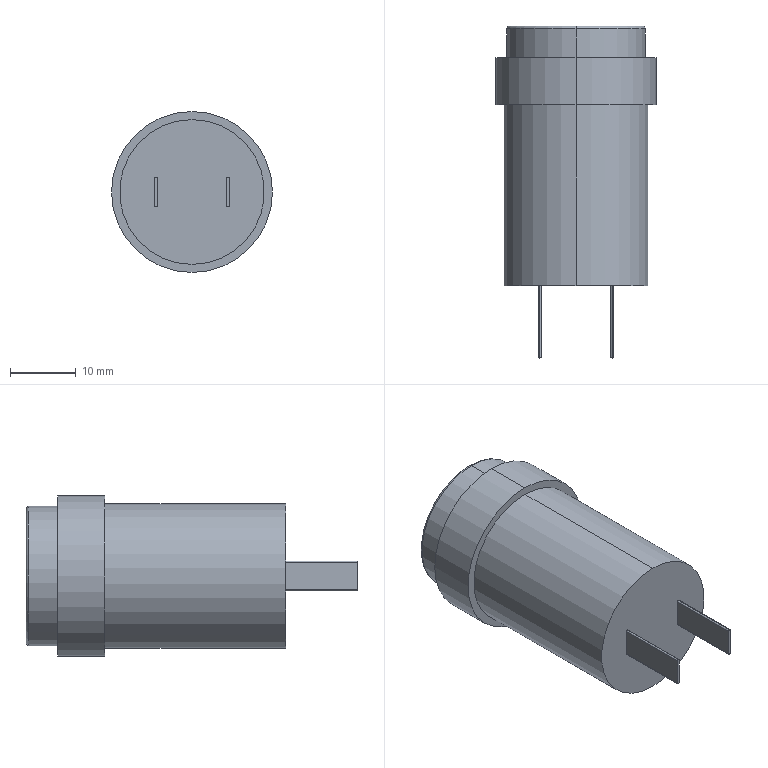Part | SolidWorks | features BaseBody 1 | 1 solid | 24 faces | box 24.475 x 50.463 x 24.475 mm | volume 15550 mm3 | cylinder 12 | plane 10 | torus 2 | commonest cylinder face diameters 0.412 x4 0.413 x2 21.175 x2 22 x2 24.475 x2
STEP:
#1=CARTESIAN_POINT('',(0.,13.6,-10.588));
#2=VERTEX_POINT('',#1);
#3=CARTESIAN_POINT('',(0.,13.6,10.588));
#4=VERTEX_POINT('',#3);
#5=CARTESIAN_POINT('',(0.,13.6,0.));
#6=DIRECTION('',(0.,-1.,0.));
#7=DIRECTION('',(0.,0.,1.));
#8=AXIS2_PLACEMENT_3D('',#5,#6,#7);
#9=CIRCLE('',#8,10.588);
#10=EDGE_CURVE('',#2,#4,#9,.T.);
#11=ORIENTED_EDGE('',*,*,#10,.F.);
#12=CARTESIAN_POINT('',(0.,14.012,-10.175));
#13=VERTEX_POINT('',#12);
#14=CARTESIAN_POINT('',(0.,13.6,-10.175));
#15=DIRECTION('',(1.,0.,0.));
#16=DIRECTION('',(0.,0.,-1.));
#17=AXIS2_PLACEMENT_3D('',#14,#15,#16);
#18=CIRCLE('',#17,0.4125);
#19=EDGE_CURVE('',#2,#13,#18,.T.);
#20=ORIENTED_EDGE('',*,*,#19,.T.);
#21=CARTESIAN_POINT('',(0.,14.012,10.175));
#22=VERTEX_POINT('',#21);
#23=CARTESIAN_POINT('',(0.,14.012,0.));
#24=DIRECTION('',(0.,1.,0.));
#25=DIRECTION('',(0.,0.,1.));
#26=AXIS2_PLACEMENT_3D('',#23,#24,#25);
#27=CIRCLE('',#26,10.175);
#28=EDGE_CURVE('',#22,#13,#27,.T.);
#29=ORIENTED_EDGE('',*,*,#28,.F.);
#30=CARTESIAN_POINT('',(0.,13.6,10.175));
#31=DIRECTION('',(-1.,0.,0.));
#32=DIRECTION('',(0.,0.,1.));
#33=AXIS2_PLACEMENT_3D('',#30,#31,#32);
#34=CIRCLE('',#33,0.4125);
#35=EDGE_CURVE('',#4,#22,#34,.T.);
#36=ORIENTED_EDGE('',*,*,#35,.F.);
#37=EDGE_LOOP('',(#11,#20,#29,#36));
#38=FACE_OUTER_BOUND('',#37,.T.);
#39=CARTESIAN_POINT('',(0.,13.6,0.));
#40=DIRECTION('',(0.,1.,0.));
#41=DIRECTION('',(0.,0.,1.));
#42=AXIS2_PLACEMENT_3D('',#39,#40,#41);
#43=TOROIDAL_SURFACE('',#42,10.175,0.4125);
#44=ADVANCED_FACE('',(#38),#43,.T.);
#45=ORIENTED_EDGE('',*,*,#10,.T.);
#46=CARTESIAN_POINT('',(0.,9.2,10.588));
#47=VERTEX_POINT('',#46);
#48=CARTESIAN_POINT('',(0.,14.012,10.588));
#49=DIRECTION('',(0.,-1.,0.));
#50=VECTOR('',#49,1000.);
#51=LINE('',#48,#50);
#52=EDGE_CURVE('',#4,#47,#51,.T.);
#53=ORIENTED_EDGE('',*,*,#52,.T.);
#54=CARTESIAN_POINT('',(0.,9.2,-10.588));
#55=VERTEX_POINT('',#54);
#56=CARTESIAN_POINT('',(0.,9.2,0.));
#57=DIRECTION('',(0.,1.,0.));
#58=DIRECTION('',(0.,0.,1.));
#59=AXIS2_PLACEMENT_3D('',#56,#57,#58);
#60=CIRCLE('',#59,10.588);
#61=EDGE_CURVE('',#47,#55,#60,.T.);
#62=ORIENTED_EDGE('',*,*,#61,.T.);
#63=CARTESIAN_POINT('',(0.,14.012,-10.588));
#64=DIRECTION('',(0.,-1.,0.));
#65=VECTOR('',#64,1000.);
#66=LINE('',#63,#65);
#67=EDGE_CURVE('',#2,#55,#66,.T.);
#68=ORIENTED_EDGE('',*,*,#67,.F.);
#69=EDGE_LOOP('',(#45,#53,#62,#68));
#70=FACE_OUTER_BOUND('',#69,.T.);
#71=CARTESIAN_POINT('',(0.,14.012,0.));
#72=DIRECTION('',(0.,-1.,0.));
#73=DIRECTION('',(0.,0.,-1.));
#74=AXIS2_PLACEMENT_3D('',#71,#72,#73);
#75=CYLINDRICAL_SURFACE('',#74,10.588);
#76=ADVANCED_FACE('',(#70),#75,.T.);
#77=CARTESIAN_POINT('',(-5.5,-36.45,2.269));
#78=VERTEX_POINT('',#77);
#79=CARTESIAN_POINT('',(-5.706,-36.45,2.062));
#80=VERTEX_POINT('',#79);
#81=CARTESIAN_POINT('',(-5.5,-36.45,2.062));
#82=DIRECTION('',(0.,-1.,0.));
#83=DIRECTION('',(0.,0.,-1.));
#84=AXIS2_PLACEMENT_3D('',#81,#82,#83);
#85=CIRCLE('',#84,0.2063);
#86=EDGE_CURVE('',#78,#80,#85,.T.);
#87=ORIENTED_EDGE('',*,*,#86,.F.);
#88=CARTESIAN_POINT('',(-5.5,-25.45,2.269));
#89=VERTEX_POINT('',#88);
#90=CARTESIAN_POINT('',(-5.5,-36.45,2.269));
#91=DIRECTION('',(0.,1.,0.));
#92=VECTOR('',#91,1000.);
#93=LINE('',#90,#92);
#94=EDGE_CURVE('',#78,#89,#93,.T.);
#95=ORIENTED_EDGE('',*,*,#94,.T.);
#96=CARTESIAN_POINT('',(-5.706,-25.45,2.062));
#97=VERTEX_POINT('',#96);
#98=CARTESIAN_POINT('',(-5.5,-25.45,2.062));
#99=DIRECTION('',(0.,-1.,0.));
#100=DIRECTION('',(0.,0.,-1.));
#101=AXIS2_PLACEMENT_3D('',#98,#99,#100);
#102=CIRCLE('',#101,0.2063);
#103=EDGE_CURVE('',#89,#97,#102,.T.);
#104=ORIENTED_EDGE('',*,*,#103,.T.);
#105=CARTESIAN_POINT('',(-5.706,-36.45,2.062));
#106=DIRECTION('',(0.,1.,0.));
#107=VECTOR('',#106,1000.);
#108=LINE('',#105,#107);
#109=EDGE_CURVE('',#80,#97,#108,.T.);
#110=ORIENTED_EDGE('',*,*,#109,.F.);
#111=EDGE_LOOP('',(#87,#95,#104,#110));
#112=FACE_OUTER_BOUND('',#111,.T.);
#113=CARTESIAN_POINT('',(-5.5,-36.45,2.062));
#114=DIRECTION('',(0.,1.,0.));
#115=DIRECTION('',(0.,0.,1.));
#116=AXIS2_PLACEMENT_3D('',#113,#114,#115);
#117=CYLINDRICAL_SURFACE('',#116,0.2062);
#118=ADVANCED_FACE('',(#112),#117,.T.);
#119=CARTESIAN_POINT('',(5.5,-36.45,2.269));
#120=VERTEX_POINT('',#119);
#121=CARTESIAN_POINT('',(5.294,-36.45,2.062));
#122=VERTEX_POINT('',#121);
#123=CARTESIAN_POINT('',(5.5,-36.45,2.062));
#124=DIRECTION('',(0.,-1.,0.));
#125=DIRECTION('',(0.,0.,-1.));
#126=AXIS2_PLACEMENT_3D('',#123,#124,#125);
#127=CIRCLE('',#126,0.2063);
#128=EDGE_CURVE('',#120,#122,#127,.T.);
#129=ORIENTED_EDGE('',*,*,#128,.F.);
#130=CARTESIAN_POINT('',(5.5,-25.45,2.269));
#131=VERTEX_POINT('',#130);
#132=CARTESIAN_POINT('',(5.5,-36.45,2.269));
#133=DIRECTION('',(0.,1.,0.));
#134=VECTOR('',#133,1000.);
#135=LINE('',#132,#134);
#136=EDGE_CURVE('',#120,#131,#135,.T.);
#137=ORIENTED_EDGE('',*,*,#136,.T.);
#138=CARTESIAN_POINT('',(5.294,-25.45,2.062));
#139=VERTEX_POINT('',#138);
#140=CARTESIAN_POINT('',(5.5,-25.45,2.062));
#141=DIRECTION('',(0.,-1.,0.));
#142=DIRECTION('',(0.,0.,-1.));
#143=AXIS2_PLACEMENT_3D('',#140,#141,#142);
#144=CIRCLE('',#143,0.2063);
#145=EDGE_CURVE('',#131,#139,#144,.T.);
#146=ORIENTED_EDGE('',*,*,#145,.T.);
#147=CARTESIAN_POINT('',(5.294,-36.45,2.062));
#148=DIRECTION('',(0.,1.,0.));
#149=VECTOR('',#148,1000.);
#150=LINE('',#147,#149);
#151=EDGE_CURVE('',#122,#139,#150,.T.);
#152=ORIENTED_EDGE('',*,*,#151,.F.);
#153=EDGE_LOOP('',(#129,#137,#146,#152));
#154=FACE_OUTER_BOUND('',#153,.T.);
#155=CARTESIAN_POINT('',(5.5,-36.45,2.062));
#156=DIRECTION('',(0.,1.,0.));
#157=DIRECTION('',(0.,0.,1.));
#158=AXIS2_PLACEMENT_3D('',#155,#156,#157);
#159=CYLINDRICAL_SURFACE('',#158,0.2062);
#160=ADVANCED_FACE('',(#154),#159,.T.);
#161=CARTESIAN_POINT('',(0.,-25.45,-11.));
#162=VERTEX_POINT('',#161);
#163=CARTESIAN_POINT('',(0.,-25.45,11.));
#164=VERTEX_POINT('',#163);
#165=CARTESIAN_POINT('',(0.,-25.45,0.));
#166=DIRECTION('',(0.,-1.,0.));
#167=DIRECTION('',(0.,0.,-1.));
#168=AXIS2_PLACEMENT_3D('',#165,#166,#167);
#169=CIRCLE('',#168,11.);
#170=EDGE_CURVE('',#162,#164,#169,.T.);
#171=ORIENTED_EDGE('',*,*,#170,.F.);
#172=CARTESIAN_POINT('',(0.,2.05,-11.));
#173=VERTEX_POINT('',#172);
#174=CARTESIAN_POINT('',(0.,-25.45,-11.));
#175=DIRECTION('',(0.,1.,0.));
#176=VECTOR('',#175,1000.);
#177=LINE('',#174,#176);
#178=EDGE_CURVE('',#162,#173,#177,.T.);
#179=ORIENTED_EDGE('',*,*,#178,.T.);
#180=CARTESIAN_POINT('',(0.,2.05,11.));
#181=VERTEX_POINT('',#180);
#182=CARTESIAN_POINT('',(0.,2.05,0.));
#183=DIRECTION('',(0.,-1.,0.));
#184=DIRECTION('',(0.,0.,1.));
#185=AXIS2_PLACEMENT_3D('',#182,#183,#184);
#186=CIRCLE('',#185,11.);
#187=EDGE_CURVE('',#173,#181,#186,.T.);
#188=ORIENTED_EDGE('',*,*,#187,.T.);
#189=CARTESIAN_POINT('',(0.,-25.45,11.));
#190=DIRECTION('',(0.,1.,0.));
#191=VECTOR('',#190,1000.);
#192=LINE('',#189,#191);
#193=EDGE_CURVE('',#164,#181,#192,.T.);
#194=ORIENTED_EDGE('',*,*,#193,.F.);
#195=EDGE_LOOP('',(#171,#179,#188,#194));
#196=FACE_OUTER_BOUND('',#195,.T.);
#197=CARTESIAN_POINT('',(0.,-25.45,0.));
#198=DIRECTION('',(0.,1.,0.));
#199=DIRECTION('',(0.,0.,1.));
#200=AXIS2_PLACEMENT_3D('',#197,#198,#199);
#201=CYLINDRICAL_SURFACE('',#200,11.);
#202=ADVANCED_FACE('',(#196),#201,.T.);
#203=CARTESIAN_POINT('',(0.,9.2,12.238));
#204=VERTEX_POINT('',#203);
#205=CARTESIAN_POINT('',(0.,9.2,-12.238));
#206=VERTEX_POINT('',#205);
#207=CARTESIAN_POINT('',(0.,9.2,0.));
#208=DIRECTION('',(0.,1.,0.));
#209=DIRECTION('',(0.,0.,1.));
#210=AXIS2_PLACEMENT_3D('',#207,#208,#209);
#211=CIRCLE('',#210,12.238);
#212=EDGE_CURVE('',#204,#206,#211,.T.);
#213=ORIENTED_EDGE('',*,*,#212,.F.);
#214=CARTESIAN_POINT('',(0.,2.05,12.238));
#215=VERTEX_POINT('',#214);
#216=CARTESIAN_POINT('',(0.,9.2,12.238));
#217=DIRECTION('',(0.,-1.,0.));
#218=VECTOR('',#217,1000.);
#219=LINE('',#216,#218);
#220=EDGE_CURVE('',#204,#215,#219,.T.);
#221=ORIENTED_EDGE('',*,*,#220,.T.);
#222=CARTESIAN_POINT('',(0.,2.05,-12.238));
#223=VERTEX_POINT('',#222);
#224=CARTESIAN_POINT('',(0.,2.05,0.));
#225=DIRECTION('',(0.,1.,0.));
#226=DIRECTION('',(0.,0.,1.));
#227=AXIS2_PLACEMENT_3D('',#224,#225,#226);
#228=CIRCLE('',#227,12.238);
#229=EDGE_CURVE('',#215,#223,#228,.T.);
#230=ORIENTED_EDGE('',*,*,#229,.T.);
#231=CARTESIAN_POINT('',(0.,9.2,-12.238));
#232=DIRECTION('',(0.,-1.,0.));
#233=VECTOR('',#232,1000.);
#234=LINE('',#231,#233);
#235=EDGE_CURVE('',#206,#223,#234,.T.);
#236=ORIENTED_EDGE('',*,*,#235,.F.);
#237=EDGE_LOOP('',(#213,#221,#230,#236));
#238=FACE_OUTER_BOUND('',#237,.T.);
#239=CARTESIAN_POINT('',(0.,9.2,0.));
#240=DIRECTION('',(0.,-1.,0.));
#241=DIRECTION('',(0.,0.,-1.));
#242=AXIS2_PLACEMENT_3D('',#239,#240,#241);
#243=CYLINDRICAL_SURFACE('',#242,12.238);
#244=ADVANCED_FACE('',(#238),#243,.T.);
#245=CARTESIAN_POINT('',(0.,9.2,0.));
#246=DIRECTION('',(0.,1.,0.));
#247=DIRECTION('',(0.,0.,1.));
#248=AXIS2_PLACEMENT_3D('',#245,#246,#247);
#249=CIRCLE('',#248,12.238);
#250=EDGE_CURVE('',#206,#204,#249,.T.);
#251=ORIENTED_EDGE('',*,*,#250,.T.);
#252=ORIENTED_EDGE('',*,*,#212,.T.);
#253=EDGE_LOOP('',(#251,#252));
#254=FACE_OUTER_BOUND('',#253,.T.);
#255=CARTESIAN_POINT('',(0.,9.2,0.));
#256=DIRECTION('',(0.,1.,0.));
#257=DIRECTION('',(0.,0.,1.));
#258=AXIS2_PLACEMENT_3D('',#255,#256,#257);
#259=CIRCLE('',#258,10.588);
#260=EDGE_CURVE('',#55,#47,#259,.T.);
#261=ORIENTED_EDGE('',*,*,#260,.F.);
#262=ORIENTED_EDGE('',*,*,#61,.F.);
#263=EDGE_LOOP('',(#261,#262));
#264=FACE_BOUND('',#263,.T.);
#265=CARTESIAN_POINT('',(0.,9.2,0.));
#266=DIRECTION('',(0.,1.,0.));
#267=DIRECTION('',(0.,0.,1.));
#268=AXIS2_PLACEMENT_3D('',#265,#266,#267);
#269=PLANE('',#268);
#270=ADVANCED_FACE('',(#254,#264),#269,.T.);
#271=CARTESIAN_POINT('',(5.294,-25.45,-2.062));
#272=VERTEX_POINT('',#271);
#273=CARTESIAN_POINT('',(5.294,-25.45,2.062));
#274=DIRECTION('',(0.,0.,-1.));
#275=VECTOR('',#274,1000.);
#276=LINE('',#273,#275);
#277=EDGE_CURVE('',#139,#272,#276,.T.);
#278=ORIENTED_EDGE('',*,*,#277,.F.);
#279=ORIENTED_EDGE('',*,*,#145,.F.);
#280=CARTESIAN_POINT('',(5.706,-25.45,2.062));
#281=VERTEX_POINT('',#280);
#282=CARTESIAN_POINT('',(5.5,-25.45,2.062));
#283=DIRECTION('',(0.,-1.,0.));
#284=DIRECTION('',(0.,0.,-1.));
#285=AXIS2_PLACEMENT_3D('',#282,#283,#284);
#286=CIRCLE('',#285,0.2063);
#287=EDGE_CURVE('',#281,#131,#286,.T.);
#288=ORIENTED_EDGE('',*,*,#287,.F.);
#289=CARTESIAN_POINT('',(5.706,-25.45,-2.062));
#290=VERTEX_POINT('',#289);
#291=CARTESIAN_POINT('',(5.706,-25.45,2.062));
#292=DIRECTION('',(0.,0.,1.));
#293=VECTOR('',#292,1000.);
#294=LINE('',#291,#293);
#295=EDGE_CURVE('',#290,#281,#294,.T.);
#296=ORIENTED_EDGE('',*,*,#295,.F.);
#297=CARTESIAN_POINT('',(5.5,-25.45,-2.062));
#298=DIRECTION('',(0.,-1.,0.));
#299=DIRECTION('',(0.,0.,-1.));
#300=AXIS2_PLACEMENT_3D('',#297,#298,#299);
#301=CIRCLE('',#300,0.2062);
#302=EDGE_CURVE('',#272,#290,#301,.T.);
#303=ORIENTED_EDGE('',*,*,#302,.F.);
#304=EDGE_LOOP('',(#278,#279,#288,#296,#303));
#305=FACE_BOUND('',#304,.T.);
#306=CARTESIAN_POINT('',(0.,-25.45,0.));
#307=DIRECTION('',(0.,-1.,0.));
#308=DIRECTION('',(0.,0.,-1.));
#309=AXIS2_PLACEMENT_3D('',#306,#307,#308);
#310=CIRCLE('',#309,11.);
#311=EDGE_CURVE('',#164,#162,#310,.T.);
#312=ORIENTED_EDGE('',*,*,#311,.T.);
#313=ORIENTED_EDGE('',*,*,#170,.T.);
#314=EDGE_LOOP('',(#312,#313));
#315=FACE_OUTER_BOUND('',#314,.T.);
#316=CARTESIAN_POINT('',(-5.706,-25.45,-2.062));
#317=VERTEX_POINT('',#316);
#318=CARTESIAN_POINT('',(-5.706,-25.45,2.062));
#319=DIRECTION('',(0.,0.,-1.));
#320=VECTOR('',#319,1000.);
#321=LINE('',#318,#320);
#322=EDGE_CURVE('',#97,#317,#321,.T.);
#323=ORIENTED_EDGE('',*,*,#322,.F.);
#324=ORIENTED_EDGE('',*,*,#103,.F.);
#325=CARTESIAN_POINT('',(-5.294,-25.45,2.062));
#326=VERTEX_POINT('',#325);
#327=CARTESIAN_POINT('',(-5.5,-25.45,2.062));
#328=DIRECTION('',(0.,-1.,0.));
#329=DIRECTION('',(0.,0.,-1.));
#330=AXIS2_PLACEMENT_3D('',#327,#328,#329);
#331=CIRCLE('',#330,0.2063);
#332=EDGE_CURVE('',#326,#89,#331,.T.);
#333=ORIENTED_EDGE('',*,*,#332,.F.);
#334=CARTESIAN_POINT('',(-5.294,-25.45,-2.062));
#335=VERTEX_POINT('',#334);
#336=CARTESIAN_POINT('',(-5.294,-25.45,2.062));
#337=DIRECTION('',(0.,0.,1.));
#338=VECTOR('',#337,1000.);
#339=LINE('',#336,#338);
#340=EDGE_CURVE('',#335,#326,#339,.T.);
#341=ORIENTED_EDGE('',*,*,#340,.F.);
#342=CARTESIAN_POINT('',(-5.5,-25.45,-2.062));
#343=DIRECTION('',(0.,-1.,0.));
#344=DIRECTION('',(0.,0.,-1.));
#345=AXIS2_PLACEMENT_3D('',#342,#343,#344);
#346=CIRCLE('',#345,0.2062);
#347=EDGE_CURVE('',#317,#335,#346,.T.);
#348=ORIENTED_EDGE('',*,*,#347,.F.);
#349=EDGE_LOOP('',(#323,#324,#333,#341,#348));
#350=FACE_BOUND('',#349,.T.);
#351=CARTESIAN_POINT('',(0.,-25.45,0.));
#352=DIRECTION('',(0.,-1.,0.));
#353=DIRECTION('',(0.,0.,-1.));
#354=AXIS2_PLACEMENT_3D('',#351,#352,#353);
#355=PLANE('',#354);
#356=ADVANCED_FACE('',(#305,#315,#350),#355,.T.);
#357=CARTESIAN_POINT('',(0.,2.05,0.));
#358=DIRECTION('',(0.,1.,0.));
#359=DIRECTION('',(0.,0.,1.));
#360=AXIS2_PLACEMENT_3D('',#357,#358,#359);
#361=CIRCLE('',#360,12.238);
#362=EDGE_CURVE('',#223,#215,#361,.T.);
#363=ORIENTED_EDGE('',*,*,#362,.F.);
#364=ORIENTED_EDGE('',*,*,#229,.F.);
#365=EDGE_LOOP('',(#363,#364));
#366=FACE_OUTER_BOUND('',#365,.T.);
#367=CARTESIAN_POINT('',(0.,2.05,0.));
#368=DIRECTION('',(0.,-1.,0.));
#369=DIRECTION('',(0.,0.,1.));
#370=AXIS2_PLACEMENT_3D('',#367,#368,#369);
#371=CIRCLE('',#370,11.);
#372=EDGE_CURVE('',#181,#173,#371,.T.);
#373=ORIENTED_EDGE('',*,*,#372,.F.);
#374=ORIENTED_EDGE('',*,*,#187,.F.);
#375=EDGE_LOOP('',(#373,#374));
#376=FACE_BOUND('',#375,.T.);
#377=CARTESIAN_POINT('',(0.,2.05,0.));
#378=DIRECTION('',(0.,1.,0.));
#379=DIRECTION('',(0.,0.,1.));
#380=AXIS2_PLACEMENT_3D('',#377,#378,#379);
#381=PLANE('',#380);
#382=ADVANCED_FACE('',(#366,#376),#381,.F.);
#383=ORIENTED_EDGE('',*,*,#220,.F.);
#384=ORIENTED_EDGE('',*,*,#250,.F.);
#385=ORIENTED_EDGE('',*,*,#235,.T.);
#386=ORIENTED_EDGE('',*,*,#362,.T.);
#387=EDGE_LOOP('',(#383,#384,#385,#386));
#388=FACE_OUTER_BOUND('',#387,.T.);
#389=CARTESIAN_POINT('',(0.,9.2,0.));
#390=DIRECTION('',(0.,-1.,0.));
#391=DIRECTION('',(0.,0.,-1.));
#392=AXIS2_PLACEMENT_3D('',#389,#390,#391);
#393=CYLINDRICAL_SURFACE('',#392,12.238);
#394=ADVANCED_FACE('',(#388),#393,.T.);
#395=ORIENTED_EDGE('',*,*,#178,.F.);
#396=ORIENTED_EDGE('',*,*,#311,.F.);
#397=ORIENTED_EDGE('',*,*,#193,.T.);
#398=ORIENTED_EDGE('',*,*,#372,.T.);
#399=EDGE_LOOP('',(#395,#396,#397,#398));
#400=FACE_OUTER_BOUND('',#399,.T.);
#401=CARTESIAN_POINT('',(0.,-25.45,0.));
#402=DIRECTION('',(0.,1.,0.));
#403=DIRECTION('',(0.,0.,1.));
#404=AXIS2_PLACEMENT_3D('',#401,#402,#403);
#405=CYLINDRICAL_SURFACE('',#404,11.);
#406=ADVANCED_FACE('',(#400),#405,.T.);
#407=ORIENTED_EDGE('',*,*,#136,.F.);
#408=CARTESIAN_POINT('',(5.706,-36.45,2.062));
#409=VERTEX_POINT('',#408);
#410=CARTESIAN_POINT('',(5.5,-36.45,2.062));
#411=DIRECTION('',(0.,-1.,0.));
#412=DIRECTION('',(0.,0.,-1.));
#413=AXIS2_PLACEMENT_3D('',#410,#411,#412);
#414=CIRCLE('',#413,0.2063);
#415=EDGE_CURVE('',#409,#120,#414,.T.);
#416=ORIENTED_EDGE('',*,*,#415,.F.);
#417=CARTESIAN_POINT('',(5.706,-36.45,2.062));
#418=DIRECTION('',(0.,1.,0.));
#419=VECTOR('',#418,1000.);
#420=LINE('',#417,#419);
#421=EDGE_CURVE('',#409,#281,#420,.T.);
#422=ORIENTED_EDGE('',*,*,#421,.T.);
#423=ORIENTED_EDGE('',*,*,#287,.T.);
#424=EDGE_LOOP('',(#407,#416,#422,#423));
#425=FACE_OUTER_BOUND('',#424,.T.);
#426=CARTESIAN_POINT('',(5.5,-36.45,2.062));
#427=DIRECTION('',(0.,1.,0.));
#428=DIRECTION('',(0.,0.,1.));
#429=AXIS2_PLACEMENT_3D('',#426,#427,#428);
#430=CYLINDRICAL_SURFACE('',#429,0.2062);
#431=ADVANCED_FACE('',(#425),#430,.T.);
#432=ORIENTED_EDGE('',*,*,#277,.T.);
#433=CARTESIAN_POINT('',(5.294,-36.45,-2.062));
#434=VERTEX_POINT('',#433);
#435=CARTESIAN_POINT('',(5.294,-36.45,-2.062));
#436=DIRECTION('',(0.,1.,0.));
#437=VECTOR('',#436,1000.);
#438=LINE('',#435,#437);
#439=EDGE_CURVE('',#434,#272,#438,.T.);
#440=ORIENTED_EDGE('',*,*,#439,.F.);
#441=CARTESIAN_POINT('',(5.294,-36.45,2.062));
#442=DIRECTION('',(0.,0.,-1.));
#443=VECTOR('',#442,1000.);
#444=LINE('',#441,#443);
#445=EDGE_CURVE('',#122,#434,#444,.T.);
#446=ORIENTED_EDGE('',*,*,#445,.F.);
#447=ORIENTED_EDGE('',*,*,#151,.T.);
#448=EDGE_LOOP('',(#432,#440,#446,#447));
#449=FACE_OUTER_BOUND('',#448,.T.);
#450=CARTESIAN_POINT('',(5.294,-36.45,2.062));
#451=DIRECTION('',(1.,0.,0.));
#452=DIRECTION('',(0.,0.,-1.));
#453=AXIS2_PLACEMENT_3D('',#450,#451,#452);
#454=PLANE('',#453);
#455=ADVANCED_FACE('',(#449),#454,.F.);
#456=ORIENTED_EDGE('',*,*,#302,.T.);
#457=CARTESIAN_POINT('',(5.706,-36.45,-2.062));
#458=VERTEX_POINT('',#457);
#459=CARTESIAN_POINT('',(5.706,-36.45,-2.062));
#460=DIRECTION('',(0.,1.,0.));
#461=VECTOR('',#460,1000.);
#462=LINE('',#459,#461);
#463=EDGE_CURVE('',#458,#290,#462,.T.);
#464=ORIENTED_EDGE('',*,*,#463,.F.);
#465=CARTESIAN_POINT('',(5.5,-36.45,-2.062));
#466=DIRECTION('',(0.,-1.,0.));
#467=DIRECTION('',(0.,0.,-1.));
#468=AXIS2_PLACEMENT_3D('',#465,#466,#467);
#469=CIRCLE('',#468,0.2062);
#470=EDGE_CURVE('',#434,#458,#469,.T.);
#471=ORIENTED_EDGE('',*,*,#470,.F.);
#472=ORIENTED_EDGE('',*,*,#439,.T.);
#473=EDGE_LOOP('',(#456,#464,#471,#472));
#474=FACE_OUTER_BOUND('',#473,.T.);
#475=CARTESIAN_POINT('',(5.5,-36.45,-2.062));
#476=DIRECTION('',(0.,1.,0.));
#477=DIRECTION('',(0.,0.,1.));
#478=AXIS2_PLACEMENT_3D('',#475,#476,#477);
#479=CYLINDRICAL_SURFACE('',#478,0.2063);
#480=ADVANCED_FACE('',(#474),#479,.T.);
#481=ORIENTED_EDGE('',*,*,#295,.T.);
#482=ORIENTED_EDGE('',*,*,#421,.F.);
#483=CARTESIAN_POINT('',(5.706,-36.45,2.062));
#484=DIRECTION('',(0.,0.,1.));
#485=VECTOR('',#484,1000.);
#486=LINE('',#483,#485);
#487=EDGE_CURVE('',#458,#409,#486,.T.);
#488=ORIENTED_EDGE('',*,*,#487,.F.);
#489=ORIENTED_EDGE('',*,*,#463,.T.);
#490=EDGE_LOOP('',(#481,#482,#488,#489));
#491=FACE_OUTER_BOUND('',#490,.T.);
#492=CARTESIAN_POINT('',(5.706,-36.45,2.062));
#493=DIRECTION('',(-1.,0.,0.));
#494=DIRECTION('',(0.,0.,1.));
#495=AXIS2_PLACEMENT_3D('',#492,#493,#494);
#496=PLANE('',#495);
#497=ADVANCED_FACE('',(#491),#496,.F.);
#498=ORIENTED_EDGE('',*,*,#415,.T.);
#499=ORIENTED_EDGE('',*,*,#128,.T.);
#500=ORIENTED_EDGE('',*,*,#445,.T.);
#501=ORIENTED_EDGE('',*,*,#470,.T.);
#502=ORIENTED_EDGE('',*,*,#487,.T.);
#503=EDGE_LOOP('',(#498,#499,#500,#501,#502));
#504=FACE_OUTER_BOUND('',#503,.T.);
#505=CARTESIAN_POINT('',(5.5,-36.45,2.062));
#506=DIRECTION('',(0.,-1.,0.));
#507=DIRECTION('',(0.,0.,-1.));
#508=AXIS2_PLACEMENT_3D('',#505,#506,#507);
#509=PLANE('',#508);
#510=ADVANCED_FACE('',(#504),#509,.T.);
#511=ORIENTED_EDGE('',*,*,#94,.F.);
#512=CARTESIAN_POINT('',(-5.294,-36.45,2.062));
#513=VERTEX_POINT('',#512);
#514=CARTESIAN_POINT('',(-5.5,-36.45,2.062));
#515=DIRECTION('',(0.,-1.,0.));
#516=DIRECTION('',(0.,0.,-1.));
#517=AXIS2_PLACEMENT_3D('',#514,#515,#516);
#518=CIRCLE('',#517,0.2063);
#519=EDGE_CURVE('',#513,#78,#518,.T.);
#520=ORIENTED_EDGE('',*,*,#519,.F.);
#521=CARTESIAN_POINT('',(-5.294,-36.45,2.062));
#522=DIRECTION('',(0.,1.,0.));
#523=VECTOR('',#522,1000.);
#524=LINE('',#521,#523);
#525=EDGE_CURVE('',#513,#326,#524,.T.);
#526=ORIENTED_EDGE('',*,*,#525,.T.);
#527=ORIENTED_EDGE('',*,*,#332,.T.);
#528=EDGE_LOOP('',(#511,#520,#526,#527));
#529=FACE_OUTER_BOUND('',#528,.T.);
#530=CARTESIAN_POINT('',(-5.5,-36.45,2.062));
#531=DIRECTION('',(0.,1.,0.));
#532=DIRECTION('',(0.,0.,1.));
#533=AXIS2_PLACEMENT_3D('',#530,#531,#532);
#534=CYLINDRICAL_SURFACE('',#533,0.2062);
#535=ADVANCED_FACE('',(#529),#534,.T.);
#536=ORIENTED_EDGE('',*,*,#322,.T.);
#537=CARTESIAN_POINT('',(-5.706,-36.45,-2.062));
#538=VERTEX_POINT('',#537);
#539=CARTESIAN_POINT('',(-5.706,-36.45,-2.062));
#540=DIRECTION('',(0.,1.,0.));
#541=VECTOR('',#540,1000.);
#542=LINE('',#539,#541);
#543=EDGE_CURVE('',#538,#317,#542,.T.);
#544=ORIENTED_EDGE('',*,*,#543,.F.);
#545=CARTESIAN_POINT('',(-5.706,-36.45,2.062));
#546=DIRECTION('',(0.,0.,-1.));
#547=VECTOR('',#546,1000.);
#548=LINE('',#545,#547);
#549=EDGE_CURVE('',#80,#538,#548,.T.);
#550=ORIENTED_EDGE('',*,*,#549,.F.);
#551=ORIENTED_EDGE('',*,*,#109,.T.);
#552=EDGE_LOOP('',(#536,#544,#550,#551));
#553=FACE_OUTER_BOUND('',#552,.T.);
#554=CARTESIAN_POINT('',(-5.706,-36.45,2.062));
#555=DIRECTION('',(1.,0.,0.));
#556=DIRECTION('',(0.,0.,-1.));
#557=AXIS2_PLACEMENT_3D('',#554,#555,#556);
#558=PLANE('',#557);
#559=ADVANCED_FACE('',(#553),#558,.F.);
#560=ORIENTED_EDGE('',*,*,#347,.T.);
#561=CARTESIAN_POINT('',(-5.294,-36.45,-2.062));
#562=VERTEX_POINT('',#561);
#563=CARTESIAN_POINT('',(-5.294,-36.45,-2.062));
#564=DIRECTION('',(0.,1.,0.));
#565=VECTOR('',#564,1000.);
#566=LINE('',#563,#565);
#567=EDGE_CURVE('',#562,#335,#566,.T.);
#568=ORIENTED_EDGE('',*,*,#567,.F.);
#569=CARTESIAN_POINT('',(-5.5,-36.45,-2.062));
#570=DIRECTION('',(0.,-1.,0.));
#571=DIRECTION('',(0.,0.,-1.));
#572=AXIS2_PLACEMENT_3D('',#569,#570,#571);
#573=CIRCLE('',#572,0.2062);
#574=EDGE_CURVE('',#538,#562,#573,.T.);
#575=ORIENTED_EDGE('',*,*,#574,.F.);
#576=ORIENTED_EDGE('',*,*,#543,.T.);
#577=EDGE_LOOP('',(#560,#568,#575,#576));
#578=FACE_OUTER_BOUND('',#577,.T.);
#579=CARTESIAN_POINT('',(-5.5,-36.45,-2.062));
#580=DIRECTION('',(0.,1.,0.));
#581=DIRECTION('',(0.,0.,1.));
#582=AXIS2_PLACEMENT_3D('',#579,#580,#581);
#583=CYLINDRICAL_SURFACE('',#582,0.2063);
#584=ADVANCED_FACE('',(#578),#583,.T.);
#585=ORIENTED_EDGE('',*,*,#340,.T.);
#586=ORIENTED_EDGE('',*,*,#525,.F.);
#587=CARTESIAN_POINT('',(-5.294,-36.45,2.062));
#588=DIRECTION('',(0.,0.,1.));
#589=VECTOR('',#588,1000.);
#590=LINE('',#587,#589);
#591=EDGE_CURVE('',#562,#513,#590,.T.);
#592=ORIENTED_EDGE('',*,*,#591,.F.);
#593=ORIENTED_EDGE('',*,*,#567,.T.);
#594=EDGE_LOOP('',(#585,#586,#592,#593));
#595=FACE_OUTER_BOUND('',#594,.T.);
#596=CARTESIAN_POINT('',(-5.294,-36.45,2.062));
#597=DIRECTION('',(-1.,0.,0.));
#598=DIRECTION('',(0.,0.,1.));
#599=AXIS2_PLACEMENT_3D('',#596,#597,#598);
#600=PLANE('',#599);
#601=ADVANCED_FACE('',(#595),#600,.F.);
#602=ORIENTED_EDGE('',*,*,#519,.T.);
#603=ORIENTED_EDGE('',*,*,#86,.T.);
#604=ORIENTED_EDGE('',*,*,#549,.T.);
#605=ORIENTED_EDGE('',*,*,#574,.T.);
#606=ORIENTED_EDGE('',*,*,#591,.T.);
#607=EDGE_LOOP('',(#602,#603,#604,#605,#606));
#608=FACE_OUTER_BOUND('',#607,.T.);
#609=CARTESIAN_POINT('',(-5.5,-36.45,2.062));
#610=DIRECTION('',(0.,-1.,0.));
#611=DIRECTION('',(0.,0.,-1.));
#612=AXIS2_PLACEMENT_3D('',#609,#610,#611);
#613=PLANE('',#612);
#614=ADVANCED_FACE('',(#608),#613,.T.);
#615=ORIENTED_EDGE('',*,*,#52,.F.);
#616=CARTESIAN_POINT('',(0.,13.6,0.));
#617=DIRECTION('',(0.,-1.,0.));
#618=DIRECTION('',(0.,0.,1.));
#619=AXIS2_PLACEMENT_3D('',#616,#617,#618);
#620=CIRCLE('',#619,10.588);
#621=EDGE_CURVE('',#4,#2,#620,.T.);
#622=ORIENTED_EDGE('',*,*,#621,.T.);
#623=ORIENTED_EDGE('',*,*,#67,.T.);
#624=ORIENTED_EDGE('',*,*,#260,.T.);
#625=EDGE_LOOP('',(#615,#622,#623,#624));
#626=FACE_OUTER_BOUND('',#625,.T.);
#627=CARTESIAN_POINT('',(0.,14.012,0.));
#628=DIRECTION('',(0.,-1.,0.));
#629=DIRECTION('',(0.,0.,-1.));
#630=AXIS2_PLACEMENT_3D('',#627,#628,#629);
#631=CYLINDRICAL_SURFACE('',#630,10.588);
#632=ADVANCED_FACE('',(#626),#631,.T.);
#633=ORIENTED_EDGE('',*,*,#28,.T.);
#634=CARTESIAN_POINT('',(0.,14.012,0.));
#635=DIRECTION('',(0.,1.,0.));
#636=DIRECTION('',(0.,0.,1.));
#637=AXIS2_PLACEMENT_3D('',#634,#635,#636);
#638=CIRCLE('',#637,10.175);
#639=EDGE_CURVE('',#13,#22,#638,.T.);
#640=ORIENTED_EDGE('',*,*,#639,.T.);
#641=EDGE_LOOP('',(#633,#640));
#642=FACE_OUTER_BOUND('',#641,.T.);
#643=CARTESIAN_POINT('',(0.,14.012,0.));
#644=DIRECTION('',(0.,1.,0.));
#645=DIRECTION('',(0.,0.,1.));
#646=AXIS2_PLACEMENT_3D('',#643,#644,#645);
#647=PLANE('',#646);
#648=ADVANCED_FACE('',(#642),#647,.T.);
#649=ORIENTED_EDGE('',*,*,#19,.F.);
#650=ORIENTED_EDGE('',*,*,#621,.F.);
#651=ORIENTED_EDGE('',*,*,#35,.T.);
#652=ORIENTED_EDGE('',*,*,#639,.F.);
#653=EDGE_LOOP('',(#649,#650,#651,#652));
#654=FACE_OUTER_BOUND('',#653,.T.);
#655=CARTESIAN_POINT('',(0.,13.6,0.));
#656=DIRECTION('',(0.,1.,0.));
#657=DIRECTION('',(0.,0.,1.));
#658=AXIS2_PLACEMENT_3D('',#655,#656,#657);
#659=TOROIDAL_SURFACE('',#658,10.175,0.4125);
#660=ADVANCED_FACE('',(#654),#659,.T.);
#661=CLOSED_SHELL('',(#44,#76,#118,#160,#202,#244,#270,#356,#382,#394,#406,#431,#455,#480,#497,#510,#535,#559,#584,#601,#614,#632,#648,#660));
#662=MANIFOLD_SOLID_BREP('',#661);
#663=CARTESIAN_POINT('',(0.,0.,0.));
#664=DIRECTION('',(0.,0.,1.));
#665=DIRECTION('',(1.,0.,0.));
#666=AXIS2_PLACEMENT_3D('',#663,#664,#665);
#667=(LENGTH_UNIT()NAMED_UNIT(*)SI_UNIT(.MILLI.,.METRE.));
#668=UNCERTAINTY_MEASURE_WITH_UNIT(LENGTH_MEASURE(0.00001),#667,'','');
#669=(NAMED_UNIT(*)PLANE_ANGLE_UNIT()SI_UNIT($,.RADIAN.));
#670=(NAMED_UNIT(*)SI_UNIT($,.STERADIAN.)SOLID_ANGLE_UNIT());
#671=(GEOMETRIC_REPRESENTATION_CONTEXT(3)GLOBAL_UNCERTAINTY_ASSIGNED_CONTEXT((#668))GLOBAL_UNIT_ASSIGNED_CONTEXT((#667,#669,#670))REPRESENTATION_CONTEXT('',''));
#672=ADVANCED_BREP_SHAPE_REPRESENTATION('',(#662,#666),#671);